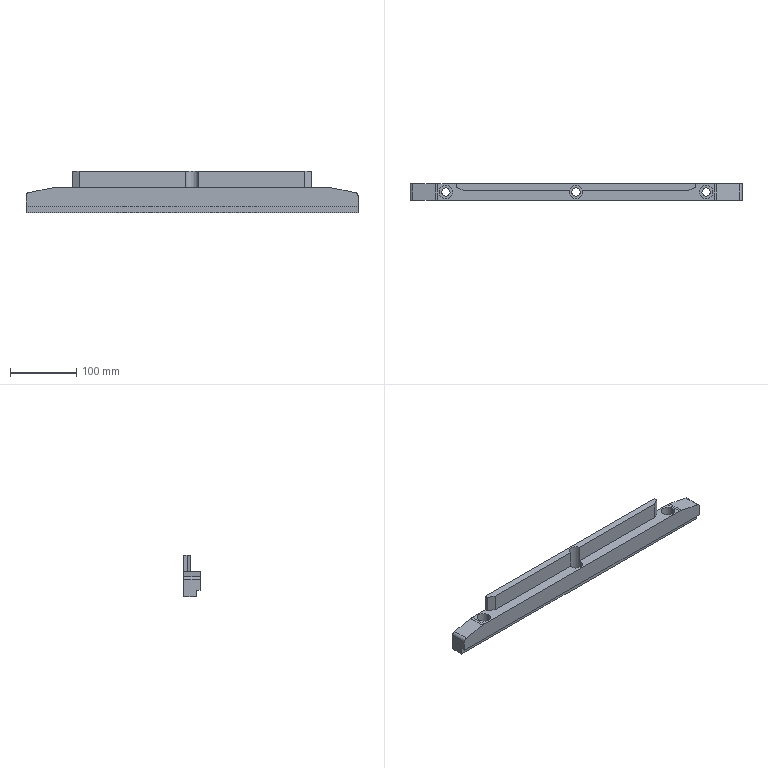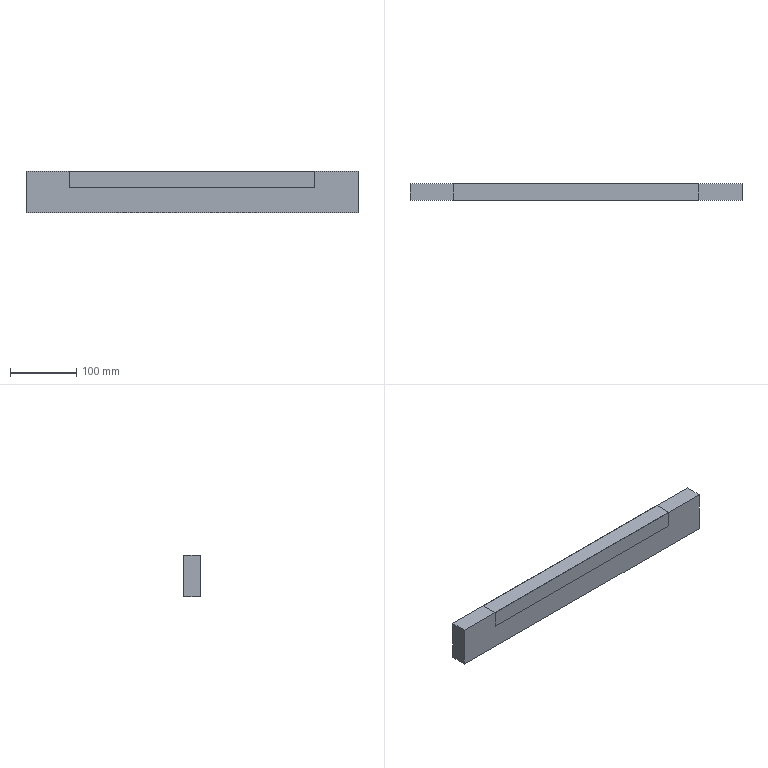CAM job | NX | 3-axis milling, drilling | part box 500 x 25 x 62.5 mm | stock box 500 x 25 x 62.5 mm
Tools:
number,name,description,diameter,corner_radius,flute_length,length,flutes
21,D12JING,Milling Tool-5 Parameters,12.0,0.0,50.0,75.0,2
2,D6A45,Milling Tool-5 Parameters,6.0,0.0,3.0,3.0,2
12,12.5ZT,Drilling Tool,12.5,0.0,35.0,50.0,2
Operations:
program,operation,operation_type,tool,method,geometry_group,spindle_rpm,surface_speed,feed_per_tooth,feed_cut,feed_plunge,cut_length_mm,path_length_mm,cut_time_min,machine_time_min
1,ADAPTIVE_MILLING,CavityMilling,D12JING,METHOD,A,9500.0,298.0,0.1579,3000.0,1000.0,7390.037,7495.735,2.464,2.475
1,HOLE_MILLING,CylinderMilling,D12JING,METHOD,A,9500.0,298.0,0.1158,2200.0,100.0,2515.173,3279.673,1.143,1.22
1,CAVITY_MILL,CavityMilling,D12JING,METHOD,A,9500.0,298.0,0.0526,1000.0,100.0,1462.56,2649.086,1.463,1.581
2,DRILLING_COPY_1,Operation,D6A45,METHOD,B,5000.0,94.0,0.025,250.0,0.0,15.3,488.646,0.0612,0.1085
2,DRILLING_COPY_COPY_1,Operation,12.5ZT,METHOD,B,1200.0,47.0,0.1042,250.0,0.0,68.266,790.567,0.2731,0.3453
2,ADAPTIVE_MILLING_COPY,CavityMilling,D12JING,METHOD,B,9500.0,298.0,0.1579,3000.0,1000.0,4137.148,5381.801,1.381,1.506
2,HOLE_MILLING_COPY_1,CylinderMilling,D12JING,METHOD,B,9500.0,298.0,0.1158,2200.0,100.0,4028.997,5192.998,1.831,1.948
2,ZLEVEL_PROFILE_COPY_COPY_1_COPY_COPY_COPY,ZLevelMilling,D12JING,METHOD,B,9500.0,298.0,0.0632,1200.0,100.0,521.091,595.091,0.4342,0.4416